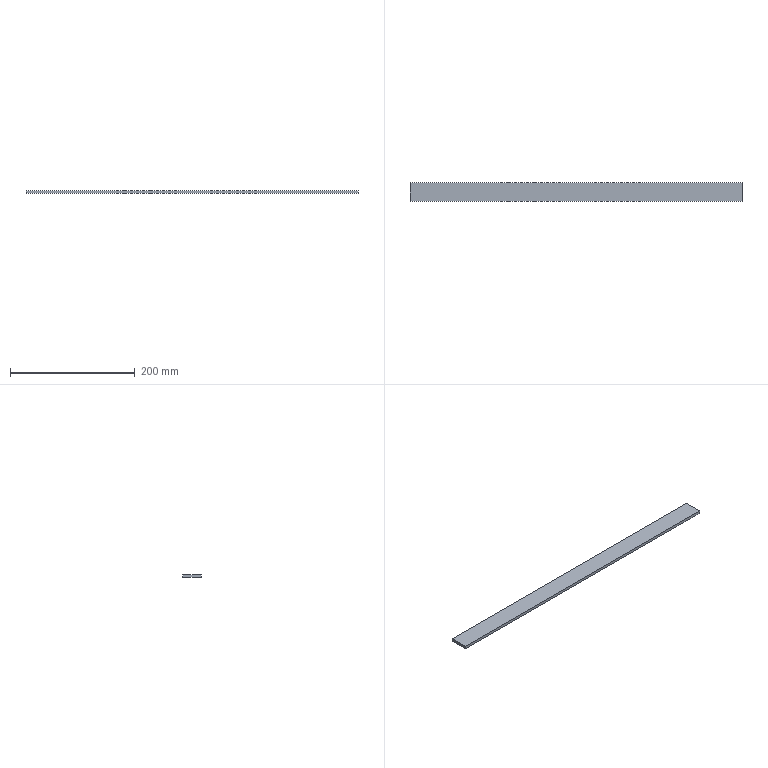Part | SolidWorks | features SplitBody 1 | 1 solid | 6 faces | box 532 x 30 x 4.6 mm | volume 73416 mm3 | plane 6
STEP:
#1=CARTESIAN_POINT('',(-57.525,282.659,-458.616));
#2=VERTEX_POINT('',#1);
#3=CARTESIAN_POINT('',(-57.525,252.659,-458.616));
#4=VERTEX_POINT('',#3);
#5=CARTESIAN_POINT('',(-57.525,282.659,-458.616));
#6=DIRECTION('',(0.,-1.,0.));
#7=VECTOR('',#6,1000.);
#8=LINE('',#5,#7);
#9=EDGE_CURVE('',#2,#4,#8,.T.);
#10=ORIENTED_EDGE('',*,*,#9,.T.);
#11=CARTESIAN_POINT('',(-57.525,252.659,-454.016));
#12=VERTEX_POINT('',#11);
#13=CARTESIAN_POINT('',(-57.525,252.659,-454.016));
#14=DIRECTION('',(0.,0.,-1.));
#15=VECTOR('',#14,1000.);
#16=LINE('',#13,#15);
#17=EDGE_CURVE('',#12,#4,#16,.T.);
#18=ORIENTED_EDGE('',*,*,#17,.F.);
#19=CARTESIAN_POINT('',(-57.525,282.659,-454.016));
#20=VERTEX_POINT('',#19);
#21=CARTESIAN_POINT('',(-57.525,282.659,-454.016));
#22=DIRECTION('',(0.,-1.,0.));
#23=VECTOR('',#22,1000.);
#24=LINE('',#21,#23);
#25=EDGE_CURVE('',#20,#12,#24,.T.);
#26=ORIENTED_EDGE('',*,*,#25,.F.);
#27=CARTESIAN_POINT('',(-57.525,282.659,-454.016));
#28=DIRECTION('',(0.,0.,-1.));
#29=VECTOR('',#28,1000.);
#30=LINE('',#27,#29);
#31=EDGE_CURVE('',#20,#2,#30,.T.);
#32=ORIENTED_EDGE('',*,*,#31,.T.);
#33=EDGE_LOOP('',(#10,#18,#26,#32));
#34=FACE_OUTER_BOUND('',#33,.T.);
#35=CARTESIAN_POINT('',(-57.525,282.659,-454.016));
#36=DIRECTION('',(1.,0.,0.));
#37=DIRECTION('',(0.,1.,0.));
#38=AXIS2_PLACEMENT_3D('',#35,#36,#37);
#39=PLANE('',#38);
#40=ADVANCED_FACE('',(#34),#39,.F.);
#41=CARTESIAN_POINT('',(474.475,252.659,-458.616));
#42=VERTEX_POINT('',#41);
#43=CARTESIAN_POINT('',(-57.525,252.659,-458.616));
#44=DIRECTION('',(1.,0.,0.));
#45=VECTOR('',#44,1000.);
#46=LINE('',#43,#45);
#47=EDGE_CURVE('',#4,#42,#46,.T.);
#48=ORIENTED_EDGE('',*,*,#47,.T.);
#49=CARTESIAN_POINT('',(474.475,252.659,-454.016));
#50=VERTEX_POINT('',#49);
#51=CARTESIAN_POINT('',(474.475,252.659,-454.016));
#52=DIRECTION('',(0.,0.,-1.));
#53=VECTOR('',#52,1000.);
#54=LINE('',#51,#53);
#55=EDGE_CURVE('',#50,#42,#54,.T.);
#56=ORIENTED_EDGE('',*,*,#55,.F.);
#57=CARTESIAN_POINT('',(-57.525,252.659,-454.016));
#58=DIRECTION('',(1.,0.,0.));
#59=VECTOR('',#58,1000.);
#60=LINE('',#57,#59);
#61=EDGE_CURVE('',#12,#50,#60,.T.);
#62=ORIENTED_EDGE('',*,*,#61,.F.);
#63=ORIENTED_EDGE('',*,*,#17,.T.);
#64=EDGE_LOOP('',(#48,#56,#62,#63));
#65=FACE_OUTER_BOUND('',#64,.T.);
#66=CARTESIAN_POINT('',(-57.525,252.659,-454.016));
#67=DIRECTION('',(0.,1.,0.));
#68=DIRECTION('',(-1.,0.,0.));
#69=AXIS2_PLACEMENT_3D('',#66,#67,#68);
#70=PLANE('',#69);
#71=ADVANCED_FACE('',(#65),#70,.F.);
#72=CARTESIAN_POINT('',(474.475,282.659,-458.616));
#73=VERTEX_POINT('',#72);
#74=CARTESIAN_POINT('',(474.475,282.659,-458.616));
#75=DIRECTION('',(0.,1.,0.));
#76=VECTOR('',#75,1000.);
#77=LINE('',#74,#76);
#78=EDGE_CURVE('',#42,#73,#77,.T.);
#79=ORIENTED_EDGE('',*,*,#78,.T.);
#80=CARTESIAN_POINT('',(474.475,282.659,-454.016));
#81=VERTEX_POINT('',#80);
#82=CARTESIAN_POINT('',(474.475,282.659,-454.016));
#83=DIRECTION('',(0.,0.,-1.));
#84=VECTOR('',#83,1000.);
#85=LINE('',#82,#84);
#86=EDGE_CURVE('',#81,#73,#85,.T.);
#87=ORIENTED_EDGE('',*,*,#86,.F.);
#88=CARTESIAN_POINT('',(474.475,282.659,-454.016));
#89=DIRECTION('',(0.,1.,0.));
#90=VECTOR('',#89,1000.);
#91=LINE('',#88,#90);
#92=EDGE_CURVE('',#50,#81,#91,.T.);
#93=ORIENTED_EDGE('',*,*,#92,.F.);
#94=ORIENTED_EDGE('',*,*,#55,.T.);
#95=EDGE_LOOP('',(#79,#87,#93,#94));
#96=FACE_OUTER_BOUND('',#95,.T.);
#97=CARTESIAN_POINT('',(474.475,282.659,-454.016));
#98=DIRECTION('',(-1.,0.,0.));
#99=DIRECTION('',(0.,0.,1.));
#100=AXIS2_PLACEMENT_3D('',#97,#98,#99);
#101=PLANE('',#100);
#102=ADVANCED_FACE('',(#96),#101,.F.);
#103=CARTESIAN_POINT('',(-57.525,282.659,-458.616));
#104=DIRECTION('',(-1.,0.,0.));
#105=VECTOR('',#104,1000.);
#106=LINE('',#103,#105);
#107=EDGE_CURVE('',#73,#2,#106,.T.);
#108=ORIENTED_EDGE('',*,*,#107,.T.);
#109=ORIENTED_EDGE('',*,*,#31,.F.);
#110=CARTESIAN_POINT('',(-57.525,282.659,-454.016));
#111=DIRECTION('',(-1.,0.,0.));
#112=VECTOR('',#111,1000.);
#113=LINE('',#110,#112);
#114=EDGE_CURVE('',#81,#20,#113,.T.);
#115=ORIENTED_EDGE('',*,*,#114,.F.);
#116=ORIENTED_EDGE('',*,*,#86,.T.);
#117=EDGE_LOOP('',(#108,#109,#115,#116));
#118=FACE_OUTER_BOUND('',#117,.T.);
#119=CARTESIAN_POINT('',(-57.525,282.659,-454.016));
#120=DIRECTION('',(0.,-1.,0.));
#121=DIRECTION('',(1.,0.,0.));
#122=AXIS2_PLACEMENT_3D('',#119,#120,#121);
#123=PLANE('',#122);
#124=ADVANCED_FACE('',(#118),#123,.F.);
#125=ORIENTED_EDGE('',*,*,#25,.T.);
#126=ORIENTED_EDGE('',*,*,#61,.T.);
#127=ORIENTED_EDGE('',*,*,#92,.T.);
#128=ORIENTED_EDGE('',*,*,#114,.T.);
#129=EDGE_LOOP('',(#125,#126,#127,#128));
#130=FACE_OUTER_BOUND('',#129,.T.);
#131=CARTESIAN_POINT('',(168.616,200.907,-454.016));
#132=DIRECTION('',(0.,0.,1.));
#133=DIRECTION('',(1.,0.,0.));
#134=AXIS2_PLACEMENT_3D('',#131,#132,#133);
#135=PLANE('',#134);
#136=ADVANCED_FACE('',(#130),#135,.T.);
#137=ORIENTED_EDGE('',*,*,#9,.F.);
#138=ORIENTED_EDGE('',*,*,#107,.F.);
#139=ORIENTED_EDGE('',*,*,#78,.F.);
#140=ORIENTED_EDGE('',*,*,#47,.F.);
#141=EDGE_LOOP('',(#137,#138,#139,#140));
#142=FACE_OUTER_BOUND('',#141,.T.);
#143=CARTESIAN_POINT('',(168.616,200.907,-458.616));
#144=DIRECTION('',(0.,0.,1.));
#145=DIRECTION('',(1.,0.,0.));
#146=AXIS2_PLACEMENT_3D('',#143,#144,#145);
#147=PLANE('',#146);
#148=ADVANCED_FACE('',(#142),#147,.F.);
#149=CLOSED_SHELL('',(#40,#71,#102,#124,#136,#148));
#150=MANIFOLD_SOLID_BREP('',#149);
#151=CARTESIAN_POINT('',(0.,0.,0.));
#152=DIRECTION('',(0.,0.,1.));
#153=DIRECTION('',(1.,0.,0.));
#154=AXIS2_PLACEMENT_3D('',#151,#152,#153);
#155=(LENGTH_UNIT()NAMED_UNIT(*)SI_UNIT(.MILLI.,.METRE.));
#156=UNCERTAINTY_MEASURE_WITH_UNIT(LENGTH_MEASURE(0.00001),#155,'','');
#157=(NAMED_UNIT(*)PLANE_ANGLE_UNIT()SI_UNIT($,.RADIAN.));
#158=(NAMED_UNIT(*)SI_UNIT($,.STERADIAN.)SOLID_ANGLE_UNIT());
#159=(GEOMETRIC_REPRESENTATION_CONTEXT(3)GLOBAL_UNCERTAINTY_ASSIGNED_CONTEXT((#156))GLOBAL_UNIT_ASSIGNED_CONTEXT((#155,#157,#158))REPRESENTATION_CONTEXT('',''));
#160=ADVANCED_BREP_SHAPE_REPRESENTATION('',(#150,#154),#159);